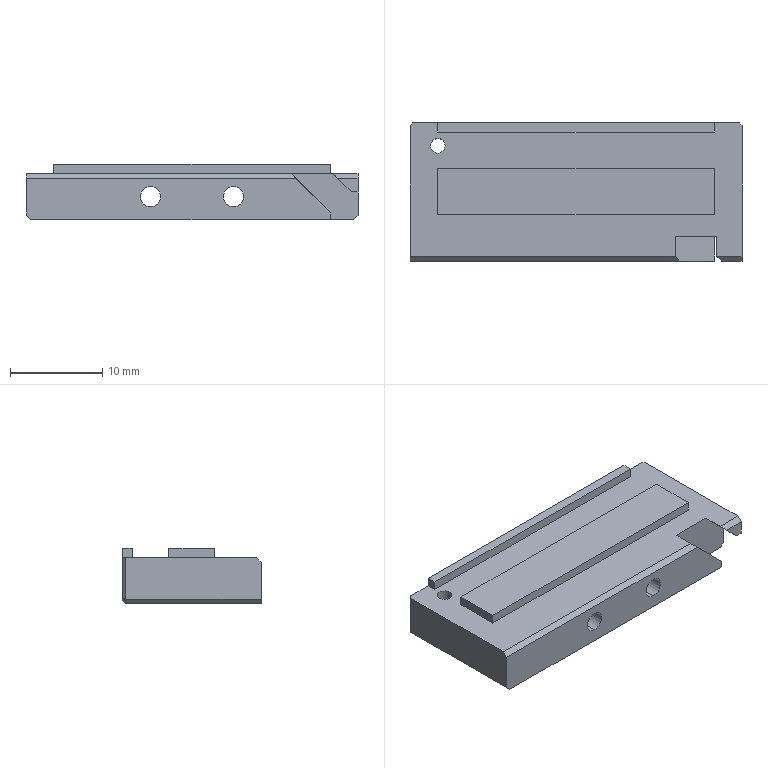Part | SolidWorks | features BaseBody 1 | 1 solid | 60 faces | box 36 x 15 x 6 mm | volume 2540 mm3 | plane 32 | cone 14 | cylinder 14 | commonest cylinder face diameters 2.2 x4 2.5 x4 4 x4 1.6 x2